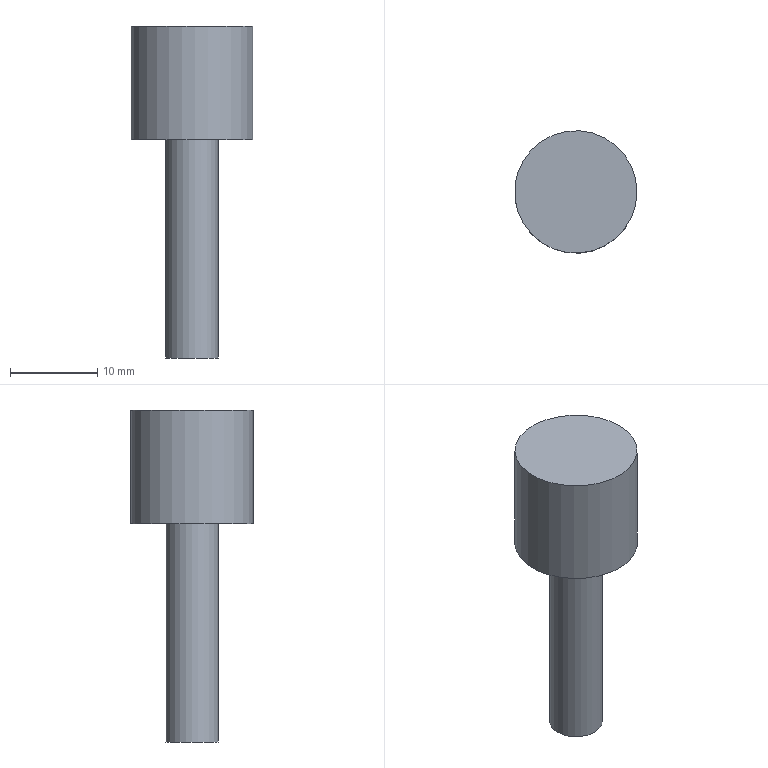Part | NX | 1 solid | 5 faces | box 14 x 14 x 38 mm | volume 2708 mm3 | plane 3 | cylinder 2 | commonest cylinder face diameters 6 x1 14 x1
STEP:
#1=CARTESIAN_POINT('',(7.,0.,0.));
#2=VERTEX_POINT('',#1);
#3=CARTESIAN_POINT('',(0.,0.,0.));
#4=DIRECTION('',(0.,0.,1.));
#5=DIRECTION('',(1.,0.,0.));
#6=AXIS2_PLACEMENT_3D('',#3,#4,#5);
#7=CIRCLE('',#6,7.);
#8=EDGE_CURVE('',#2,#2,#7,.T.);
#9=ORIENTED_EDGE('',*,*,#8,.F.);
#10=EDGE_LOOP('',(#9));
#11=FACE_BOUND('',#10,.T.);
#12=CARTESIAN_POINT('',(3.,0.,0.));
#13=VERTEX_POINT('',#12);
#14=CARTESIAN_POINT('',(0.,0.,0.));
#15=DIRECTION('',(0.,0.,1.));
#16=DIRECTION('',(1.,0.,0.));
#17=AXIS2_PLACEMENT_3D('',#14,#15,#16);
#18=CIRCLE('',#17,3.);
#19=EDGE_CURVE('',#13,#13,#18,.F.);
#20=ORIENTED_EDGE('',*,*,#19,.F.);
#21=EDGE_LOOP('',(#20));
#22=FACE_BOUND('',#21,.T.);
#23=CARTESIAN_POINT('',(0.,0.,0.));
#24=DIRECTION('',(0.,0.,1.));
#25=DIRECTION('',(1.,0.,0.));
#26=AXIS2_PLACEMENT_3D('',#23,#24,#25);
#27=PLANE('',#26);
#28=ADVANCED_FACE('',(#11,#22),#27,.F.);
#29=CARTESIAN_POINT('',(7.,0.,13.));
#30=VERTEX_POINT('',#29);
#31=CARTESIAN_POINT('',(0.,0.,13.));
#32=DIRECTION('',(0.,0.,1.));
#33=DIRECTION('',(1.,0.,0.));
#34=AXIS2_PLACEMENT_3D('',#31,#32,#33);
#35=CIRCLE('',#34,7.);
#36=EDGE_CURVE('',#30,#30,#35,.T.);
#37=ORIENTED_EDGE('',*,*,#36,.F.);
#38=EDGE_LOOP('',(#37));
#39=FACE_BOUND('',#38,.T.);
#40=ORIENTED_EDGE('',*,*,#8,.T.);
#41=EDGE_LOOP('',(#40));
#42=FACE_BOUND('',#41,.T.);
#43=CARTESIAN_POINT('',(0.,0.,13.));
#44=DIRECTION('',(0.,0.,-1.));
#45=DIRECTION('',(-1.,0.,0.));
#46=AXIS2_PLACEMENT_3D('',#43,#44,#45);
#47=CYLINDRICAL_SURFACE('',#46,7.);
#48=ADVANCED_FACE('',(#39,#42),#47,.T.);
#49=ORIENTED_EDGE('',*,*,#36,.T.);
#50=EDGE_LOOP('',(#49));
#51=FACE_BOUND('',#50,.T.);
#52=CARTESIAN_POINT('',(0.,0.,13.));
#53=DIRECTION('',(0.,0.,1.));
#54=DIRECTION('',(1.,0.,0.));
#55=AXIS2_PLACEMENT_3D('',#52,#53,#54);
#56=PLANE('',#55);
#57=ADVANCED_FACE('',(#51),#56,.T.);
#58=CARTESIAN_POINT('',(-3.,0.,-25.));
#59=VERTEX_POINT('',#58);
#60=CARTESIAN_POINT('',(0.,0.,-25.));
#61=DIRECTION('',(0.,0.,-1.));
#62=DIRECTION('',(-1.,0.,0.));
#63=AXIS2_PLACEMENT_3D('',#60,#61,#62);
#64=CIRCLE('',#63,3.);
#65=EDGE_CURVE('',#59,#59,#64,.T.);
#66=ORIENTED_EDGE('',*,*,#65,.F.);
#67=EDGE_LOOP('',(#66));
#68=FACE_BOUND('',#67,.T.);
#69=ORIENTED_EDGE('',*,*,#19,.T.);
#70=EDGE_LOOP('',(#69));
#71=FACE_BOUND('',#70,.T.);
#72=CARTESIAN_POINT('',(0.,0.,-25.));
#73=DIRECTION('',(0.,0.,1.));
#74=DIRECTION('',(1.,0.,0.));
#75=AXIS2_PLACEMENT_3D('',#72,#73,#74);
#76=CYLINDRICAL_SURFACE('',#75,3.);
#77=ADVANCED_FACE('',(#68,#71),#76,.T.);
#78=ORIENTED_EDGE('',*,*,#65,.T.);
#79=EDGE_LOOP('',(#78));
#80=FACE_BOUND('',#79,.T.);
#81=CARTESIAN_POINT('',(0.,0.,-25.));
#82=DIRECTION('',(0.,0.,-1.));
#83=DIRECTION('',(-1.,0.,0.));
#84=AXIS2_PLACEMENT_3D('',#81,#82,#83);
#85=PLANE('',#84);
#86=ADVANCED_FACE('',(#80),#85,.T.);
#87=CLOSED_SHELL('',(#28,#48,#57,#77,#86));
#88=MANIFOLD_SOLID_BREP('',#87);
#89=(LENGTH_UNIT()NAMED_UNIT(*)SI_UNIT(.MILLI.,.METRE.));
#90=UNCERTAINTY_MEASURE_WITH_UNIT(LENGTH_MEASURE(0.00001),#89,'','');
#91=(NAMED_UNIT(*)PLANE_ANGLE_UNIT()SI_UNIT($,.RADIAN.));
#92=(NAMED_UNIT(*)SI_UNIT($,.STERADIAN.)SOLID_ANGLE_UNIT());
#93=(GEOMETRIC_REPRESENTATION_CONTEXT(3)GLOBAL_UNCERTAINTY_ASSIGNED_CONTEXT((#90))GLOBAL_UNIT_ASSIGNED_CONTEXT((#89,#91,#92))REPRESENTATION_CONTEXT('',''));
#94=ADVANCED_BREP_SHAPE_REPRESENTATION('',(#88),#93);